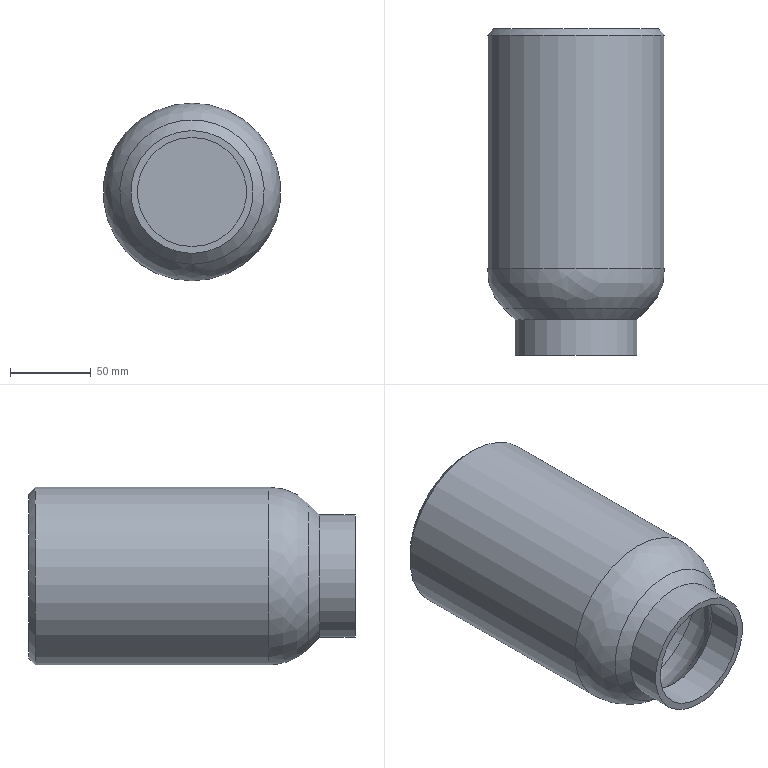Part | NX | 2 solids | 15 faces | box 110 x 202 x 110 mm | volume 227376 mm3 | plane 5 | cylinder 4 | cone 4 | spline 2 | commonest cylinder face diameters 67.515 x1 76 x1 104 x1 110 x1
STEP:
#1=CARTESIAN_POINT('',(4712.585,-22.,-359.679));
#2=VERTEX_POINT('',#1);
#3=CARTESIAN_POINT('',(4712.585,-22.,-321.679));
#4=DIRECTION('',(0.,-1.,0.));
#5=DIRECTION('',(0.,0.,-1.));
#6=AXIS2_PLACEMENT_3D('',#3,#4,#5);
#7=CIRCLE('',#6,38.);
#8=EDGE_CURVE('',#2,#2,#7,.T.);
#9=ORIENTED_EDGE('',*,*,#8,.F.);
#10=EDGE_LOOP('',(#9));
#11=FACE_BOUND('',#10,.T.);
#12=CARTESIAN_POINT('',(4712.585,0.,-359.679));
#13=VERTEX_POINT('',#12);
#14=CARTESIAN_POINT('',(4712.585,0.,-321.679));
#15=DIRECTION('',(0.,-1.,0.));
#16=DIRECTION('',(0.,0.,-1.));
#17=AXIS2_PLACEMENT_3D('',#14,#15,#16);
#18=CIRCLE('',#17,38.);
#19=EDGE_CURVE('',#13,#13,#18,.T.);
#20=ORIENTED_EDGE('',*,*,#19,.T.);
#21=EDGE_LOOP('',(#20));
#22=FACE_BOUND('',#21,.T.);
#23=CARTESIAN_POINT('',(4712.585,-22.,-321.679));
#24=DIRECTION('',(0.,1.,0.));
#25=DIRECTION('',(0.,0.,1.));
#26=AXIS2_PLACEMENT_3D('',#23,#24,#25);
#27=CYLINDRICAL_SURFACE('',#26,38.);
#28=ADVANCED_FACE('',(#11,#22),#27,.T.);
#29=CARTESIAN_POINT('',(4712.585,-22.,-355.436));
#30=VERTEX_POINT('',#29);
#31=CARTESIAN_POINT('',(4712.585,-22.,-321.679));
#32=DIRECTION('',(0.,-1.,0.));
#33=DIRECTION('',(0.,0.,-1.));
#34=AXIS2_PLACEMENT_3D('',#31,#32,#33);
#35=CIRCLE('',#34,33.757);
#36=EDGE_CURVE('',#30,#30,#35,.T.);
#37=ORIENTED_EDGE('',*,*,#36,.T.);
#38=EDGE_LOOP('',(#37));
#39=FACE_BOUND('',#38,.T.);
#40=CARTESIAN_POINT('',(4712.585,0.,-355.436));
#41=VERTEX_POINT('',#40);
#42=CARTESIAN_POINT('',(4712.585,0.,-321.679));
#43=DIRECTION('',(0.,-1.,0.));
#44=DIRECTION('',(0.,0.,-1.));
#45=AXIS2_PLACEMENT_3D('',#42,#43,#44);
#46=CIRCLE('',#45,33.757);
#47=EDGE_CURVE('',#41,#41,#46,.T.);
#48=ORIENTED_EDGE('',*,*,#47,.F.);
#49=EDGE_LOOP('',(#48));
#50=FACE_BOUND('',#49,.T.);
#51=CARTESIAN_POINT('',(4712.585,-22.,-321.679));
#52=DIRECTION('',(0.,1.,0.));
#53=DIRECTION('',(0.,0.,1.));
#54=AXIS2_PLACEMENT_3D('',#51,#52,#53);
#55=CYLINDRICAL_SURFACE('',#54,33.757);
#56=ADVANCED_FACE('',(#39,#50),#55,.F.);
#57=ORIENTED_EDGE('',*,*,#8,.T.);
#58=EDGE_LOOP('',(#57));
#59=FACE_BOUND('',#58,.T.);
#60=ORIENTED_EDGE('',*,*,#36,.F.);
#61=EDGE_LOOP('',(#60));
#62=FACE_BOUND('',#61,.T.);
#63=CARTESIAN_POINT('',(4712.585,-22.,-321.679));
#64=DIRECTION('',(0.,-1.,0.));
#65=DIRECTION('',(0.,0.,-1.));
#66=AXIS2_PLACEMENT_3D('',#63,#64,#65);
#67=PLANE('',#66);
#68=ADVANCED_FACE('',(#59,#62),#67,.T.);
#69=ORIENTED_EDGE('',*,*,#19,.F.);
#70=EDGE_LOOP('',(#69));
#71=FACE_BOUND('',#70,.T.);
#72=ORIENTED_EDGE('',*,*,#47,.T.);
#73=EDGE_LOOP('',(#72));
#74=FACE_BOUND('',#73,.T.);
#75=CARTESIAN_POINT('',(4712.585,0.,-321.679));
#76=DIRECTION('',(0.,-1.,0.));
#77=DIRECTION('',(0.,0.,-1.));
#78=AXIS2_PLACEMENT_3D('',#75,#76,#77);
#79=PLANE('',#78);
#80=ADVANCED_FACE('',(#71,#74),#79,.F.);
#81=CLOSED_SHELL('',(#28,#56,#68,#80));
#82=MANIFOLD_SOLID_BREP('',#81);
#83=CARTESIAN_POINT('',(4712.585,176.,-376.679));
#84=VERTEX_POINT('',#83);
#85=CARTESIAN_POINT('',(4712.585,176.,-321.679));
#86=DIRECTION('',(0.,-1.,0.));
#87=DIRECTION('',(0.,0.,-1.));
#88=AXIS2_PLACEMENT_3D('',#85,#86,#87);
#89=CIRCLE('',#88,55.);
#90=EDGE_CURVE('',#84,#84,#89,.T.);
#91=ORIENTED_EDGE('',*,*,#90,.T.);
#92=EDGE_LOOP('',(#91));
#93=FACE_BOUND('',#92,.T.);
#94=CARTESIAN_POINT('',(4712.585,31.497,-376.679));
#95=VERTEX_POINT('',#94);
#96=CARTESIAN_POINT('',(4712.585,31.497,-321.679));
#97=DIRECTION('',(0.,1.,0.));
#98=DIRECTION('',(0.,0.,-1.));
#99=AXIS2_PLACEMENT_3D('',#96,#97,#98);
#100=CIRCLE('',#99,55.);
#101=EDGE_CURVE('',#95,#95,#100,.T.);
#102=ORIENTED_EDGE('',*,*,#101,.T.);
#103=EDGE_LOOP('',(#102));
#104=FACE_BOUND('',#103,.T.);
#105=CARTESIAN_POINT('',(4712.585,180.,-321.679));
#106=DIRECTION('',(0.,-1.,0.));
#107=DIRECTION('',(0.,0.,-1.));
#108=AXIS2_PLACEMENT_3D('',#105,#106,#107);
#109=CYLINDRICAL_SURFACE('',#108,55.);
#110=ADVANCED_FACE('',(#93,#104),#109,.T.);
#111=CARTESIAN_POINT('',(4712.585,180.,-372.679));
#112=VERTEX_POINT('',#111);
#113=CARTESIAN_POINT('',(4712.585,180.,-321.679));
#114=DIRECTION('',(0.,1.,0.));
#115=DIRECTION('',(0.,0.,-1.));
#116=AXIS2_PLACEMENT_3D('',#113,#114,#115);
#117=CIRCLE('',#116,51.);
#118=EDGE_CURVE('',#112,#112,#117,.T.);
#119=ORIENTED_EDGE('',*,*,#118,.T.);
#120=EDGE_LOOP('',(#119));
#121=FACE_OUTER_BOUND('',#120,.T.);
#122=CARTESIAN_POINT('',(4712.585,180.,-321.679));
#123=DIRECTION('',(0.,-1.,0.));
#124=DIRECTION('',(0.,0.,-1.));
#125=AXIS2_PLACEMENT_3D('',#122,#123,#124);
#126=PLANE('',#125);
#127=ADVANCED_FACE('',(#121),#126,.F.);
#128=CARTESIAN_POINT('',(4712.585,0.,-355.436));
#129=VERTEX_POINT('',#128);
#130=CARTESIAN_POINT('',(4712.585,0.,-321.679));
#131=DIRECTION('',(0.,-1.,0.));
#132=DIRECTION('',(0.,0.,-1.));
#133=AXIS2_PLACEMENT_3D('',#130,#131,#132);
#134=CIRCLE('',#133,33.757);
#135=EDGE_CURVE('',#129,#129,#134,.T.);
#136=ORIENTED_EDGE('',*,*,#135,.F.);
#137=EDGE_LOOP('',(#136));
#138=FACE_BOUND('',#137,.T.);
#139=CARTESIAN_POINT('',(4712.585,0.,-359.679));
#140=VERTEX_POINT('',#139);
#141=CARTESIAN_POINT('',(4712.585,0.,-321.679));
#142=DIRECTION('',(0.,-1.,0.));
#143=DIRECTION('',(0.,0.,-1.));
#144=AXIS2_PLACEMENT_3D('',#141,#142,#143);
#145=CIRCLE('',#144,38.);
#146=EDGE_CURVE('',#140,#140,#145,.T.);
#147=ORIENTED_EDGE('',*,*,#146,.T.);
#148=EDGE_LOOP('',(#147));
#149=FACE_BOUND('',#148,.T.);
#150=CARTESIAN_POINT('',(4712.585,0.,-321.679));
#151=DIRECTION('',(0.,-1.,0.));
#152=DIRECTION('',(0.,0.,-1.));
#153=AXIS2_PLACEMENT_3D('',#150,#151,#152);
#154=PLANE('',#153);
#155=ADVANCED_FACE('',(#138,#149),#154,.T.);
#156=CARTESIAN_POINT('',(4712.585,6.749,-366.428));
#157=VERTEX_POINT('',#156);
#158=CARTESIAN_POINT('',(4712.585,6.749,-321.679));
#159=DIRECTION('',(0.,-1.,0.));
#160=DIRECTION('',(0.,0.,-1.));
#161=AXIS2_PLACEMENT_3D('',#158,#159,#160);
#162=CIRCLE('',#161,44.749);
#163=EDGE_CURVE('',#157,#157,#162,.T.);
#164=ORIENTED_EDGE('',*,*,#163,.T.);
#165=EDGE_LOOP('',(#164));
#166=FACE_BOUND('',#165,.T.);
#167=ORIENTED_EDGE('',*,*,#146,.F.);
#168=EDGE_LOOP('',(#167));
#169=FACE_BOUND('',#168,.T.);
#170=CARTESIAN_POINT('',(4712.585,0.,-321.679));
#171=DIRECTION('',(0.,1.,0.));
#172=DIRECTION('',(0.,0.,1.));
#173=AXIS2_PLACEMENT_3D('',#170,#171,#172);
#174=CONICAL_SURFACE('',#173,38.,45.);
#175=ADVANCED_FACE('',(#166,#169),#174,.T.);
#176=ORIENTED_EDGE('',*,*,#163,.F.);
#177=EDGE_LOOP('',(#176));
#178=FACE_BOUND('',#177,.T.);
#179=ORIENTED_EDGE('',*,*,#101,.F.);
#180=EDGE_LOOP('',(#179));
#181=FACE_BOUND('',#180,.T.);
#182=CARTESIAN_POINT('',(4712.585,6.749,-366.428));
#183=CARTESIAN_POINT('',(4802.082,6.749,-366.428));
#184=CARTESIAN_POINT('',(4802.082,6.749,-276.93));
#185=CARTESIAN_POINT('',(4712.585,6.749,-276.93));
#186=CARTESIAN_POINT('',(4623.087,6.749,-276.93));
#187=CARTESIAN_POINT('',(4623.087,6.749,-366.428));
#188=CARTESIAN_POINT('',(4712.585,6.749,-366.428));
#189=CARTESIAN_POINT('',(4712.585,13.4,-373.079));
#190=CARTESIAN_POINT('',(4815.385,13.4,-373.079));
#191=CARTESIAN_POINT('',(4815.385,13.4,-270.279));
#192=CARTESIAN_POINT('',(4712.585,13.4,-270.279));
#193=CARTESIAN_POINT('',(4609.784,13.4,-270.279));
#194=CARTESIAN_POINT('',(4609.784,13.4,-373.079));
#195=CARTESIAN_POINT('',(4712.585,13.4,-373.079));
#196=CARTESIAN_POINT('',(4712.585,22.091,-376.679));
#197=CARTESIAN_POINT('',(4822.585,22.091,-376.679));
#198=CARTESIAN_POINT('',(4822.585,22.091,-266.679));
#199=CARTESIAN_POINT('',(4712.585,22.091,-266.679));
#200=CARTESIAN_POINT('',(4602.585,22.091,-266.679));
#201=CARTESIAN_POINT('',(4602.585,22.091,-376.679));
#202=CARTESIAN_POINT('',(4712.585,22.091,-376.679));
#203=CARTESIAN_POINT('',(4712.585,31.497,-376.679));
#204=CARTESIAN_POINT('',(4822.585,31.497,-376.679));
#205=CARTESIAN_POINT('',(4822.585,31.497,-266.679));
#206=CARTESIAN_POINT('',(4712.585,31.497,-266.679));
#207=CARTESIAN_POINT('',(4602.585,31.497,-266.679));
#208=CARTESIAN_POINT('',(4602.585,31.497,-376.679));
#209=CARTESIAN_POINT('',(4712.585,31.497,-376.679));
#210=(BOUNDED_SURFACE()B_SPLINE_SURFACE(3,3,((#182,#183,#184,#185,#186,#187,#188),(#189,#190,#191,#192,#193,#194,#195),(#196,#197,#198,#199,#200,#201,#202),(#203,#204,#205,#206,#207,#208,#209)),.UNSPECIFIED.,.F.,.T.,.F.)B_SPLINE_SURFACE_WITH_KNOTS((4,4),(1,3,3,3,1),(0.,1.),(-0.5,0.,0.5,1.,1.5),.UNSPECIFIED.)GEOMETRIC_REPRESENTATION_ITEM()RATIONAL_B_SPLINE_SURFACE(((1.,0.3333,0.3333,1.,0.3333,0.3333,1.),(0.9493,0.3164,0.3164,0.9493,0.3164,0.3164,0.9493),(0.9493,0.3164,0.3164,0.9493,0.3164,0.3164,0.9493),(1.,0.3333,0.3333,1.,0.3333,0.3333,1.)))REPRESENTATION_ITEM('')SURFACE());
#211=ADVANCED_FACE('',(#178,#181),#210,.T.);
#212=ORIENTED_EDGE('',*,*,#118,.F.);
#213=EDGE_LOOP('',(#212));
#214=FACE_BOUND('',#213,.T.);
#215=ORIENTED_EDGE('',*,*,#90,.F.);
#216=EDGE_LOOP('',(#215));
#217=FACE_BOUND('',#216,.T.);
#218=CARTESIAN_POINT('',(4712.585,176.,-321.679));
#219=DIRECTION('',(0.,-1.,0.));
#220=DIRECTION('',(0.,0.,-1.));
#221=AXIS2_PLACEMENT_3D('',#218,#219,#220);
#222=CONICAL_SURFACE('',#221,55.,45.);
#223=ADVANCED_FACE('',(#214,#217),#222,.T.);
#224=CARTESIAN_POINT('',(4712.585,174.757,-373.679));
#225=VERTEX_POINT('',#224);
#226=CARTESIAN_POINT('',(4712.585,174.757,-321.679));
#227=DIRECTION('',(0.,-1.,0.));
#228=DIRECTION('',(0.,0.,-1.));
#229=AXIS2_PLACEMENT_3D('',#226,#227,#228);
#230=CIRCLE('',#229,52.);
#231=EDGE_CURVE('',#225,#225,#230,.T.);
#232=ORIENTED_EDGE('',*,*,#231,.F.);
#233=EDGE_LOOP('',(#232));
#234=FACE_BOUND('',#233,.T.);
#235=CARTESIAN_POINT('',(4712.585,31.497,-373.679));
#236=VERTEX_POINT('',#235);
#237=CARTESIAN_POINT('',(4712.585,31.497,-321.679));
#238=DIRECTION('',(0.,1.,0.));
#239=DIRECTION('',(0.,0.,-1.));
#240=AXIS2_PLACEMENT_3D('',#237,#238,#239);
#241=CIRCLE('',#240,52.);
#242=EDGE_CURVE('',#236,#236,#241,.T.);
#243=ORIENTED_EDGE('',*,*,#242,.F.);
#244=EDGE_LOOP('',(#243));
#245=FACE_BOUND('',#244,.T.);
#246=CARTESIAN_POINT('',(4712.585,180.,-321.679));
#247=DIRECTION('',(0.,-1.,0.));
#248=DIRECTION('',(0.,0.,-1.));
#249=AXIS2_PLACEMENT_3D('',#246,#247,#248);
#250=CYLINDRICAL_SURFACE('',#249,52.);
#251=ADVANCED_FACE('',(#234,#245),#250,.F.);
#252=CARTESIAN_POINT('',(4712.585,177.,-371.436));
#253=VERTEX_POINT('',#252);
#254=CARTESIAN_POINT('',(4712.585,177.,-321.679));
#255=DIRECTION('',(0.,1.,0.));
#256=DIRECTION('',(0.,0.,-1.));
#257=AXIS2_PLACEMENT_3D('',#254,#255,#256);
#258=CIRCLE('',#257,49.757);
#259=EDGE_CURVE('',#253,#253,#258,.T.);
#260=ORIENTED_EDGE('',*,*,#259,.F.);
#261=EDGE_LOOP('',(#260));
#262=FACE_OUTER_BOUND('',#261,.T.);
#263=CARTESIAN_POINT('',(4712.585,177.,-321.679));
#264=DIRECTION('',(0.,-1.,0.));
#265=DIRECTION('',(0.,0.,-1.));
#266=AXIS2_PLACEMENT_3D('',#263,#264,#265);
#267=PLANE('',#266);
#268=ADVANCED_FACE('',(#262),#267,.T.);
#269=CARTESIAN_POINT('',(4712.585,8.87,-279.051));
#270=VERTEX_POINT('',#269);
#271=CARTESIAN_POINT('',(4712.585,8.87,-321.679));
#272=DIRECTION('',(0.,-1.,0.));
#273=DIRECTION('',(0.,0.,1.));
#274=AXIS2_PLACEMENT_3D('',#271,#272,#273);
#275=CIRCLE('',#274,42.627);
#276=EDGE_CURVE('',#270,#270,#275,.T.);
#277=ORIENTED_EDGE('',*,*,#276,.F.);
#278=EDGE_LOOP('',(#277));
#279=FACE_BOUND('',#278,.T.);
#280=ORIENTED_EDGE('',*,*,#135,.T.);
#281=EDGE_LOOP('',(#280));
#282=FACE_BOUND('',#281,.T.);
#283=CARTESIAN_POINT('',(4712.585,2.121,-321.679));
#284=DIRECTION('',(0.,1.,0.));
#285=DIRECTION('',(0.,0.,1.));
#286=AXIS2_PLACEMENT_3D('',#283,#284,#285);
#287=CONICAL_SURFACE('',#286,35.879,45.);
#288=ADVANCED_FACE('',(#279,#282),#287,.F.);
#289=ORIENTED_EDGE('',*,*,#276,.T.);
#290=EDGE_LOOP('',(#289));
#291=FACE_BOUND('',#290,.T.);
#292=ORIENTED_EDGE('',*,*,#242,.T.);
#293=EDGE_LOOP('',(#292));
#294=FACE_BOUND('',#293,.T.);
#295=CARTESIAN_POINT('',(4712.585,31.497,-373.679));
#296=CARTESIAN_POINT('',(4816.585,31.497,-373.679));
#297=CARTESIAN_POINT('',(4816.585,31.497,-269.679));
#298=CARTESIAN_POINT('',(4712.585,31.497,-269.679));
#299=CARTESIAN_POINT('',(4608.585,31.497,-269.679));
#300=CARTESIAN_POINT('',(4608.585,31.497,-373.679));
#301=CARTESIAN_POINT('',(4712.585,31.497,-373.679));
#302=CARTESIAN_POINT('',(4712.585,22.897,-373.679));
#303=CARTESIAN_POINT('',(4816.585,22.897,-373.679));
#304=CARTESIAN_POINT('',(4816.585,22.897,-269.679));
#305=CARTESIAN_POINT('',(4712.585,22.897,-269.679));
#306=CARTESIAN_POINT('',(4608.585,22.897,-269.679));
#307=CARTESIAN_POINT('',(4608.585,22.897,-373.679));
#308=CARTESIAN_POINT('',(4712.585,22.897,-373.679));
#309=CARTESIAN_POINT('',(4712.585,14.951,-370.388));
#310=CARTESIAN_POINT('',(4810.002,14.951,-370.388));
#311=CARTESIAN_POINT('',(4810.002,14.951,-272.97));
#312=CARTESIAN_POINT('',(4712.585,14.951,-272.97));
#313=CARTESIAN_POINT('',(4615.167,14.951,-272.97));
#314=CARTESIAN_POINT('',(4615.167,14.951,-370.388));
#315=CARTESIAN_POINT('',(4712.585,14.951,-370.388));
#316=CARTESIAN_POINT('',(4712.585,8.87,-364.306));
#317=CARTESIAN_POINT('',(4797.84,8.87,-364.306));
#318=CARTESIAN_POINT('',(4797.84,8.87,-279.051));
#319=CARTESIAN_POINT('',(4712.585,8.87,-279.051));
#320=CARTESIAN_POINT('',(4627.33,8.87,-279.051));
#321=CARTESIAN_POINT('',(4627.33,8.87,-364.306));
#322=CARTESIAN_POINT('',(4712.585,8.87,-364.306));
#323=(BOUNDED_SURFACE()B_SPLINE_SURFACE(3,3,((#295,#296,#297,#298,#299,#300,#301),(#302,#303,#304,#305,#306,#307,#308),(#309,#310,#311,#312,#313,#314,#315),(#316,#317,#318,#319,#320,#321,#322)),.UNSPECIFIED.,.F.,.T.,.F.)B_SPLINE_SURFACE_WITH_KNOTS((4,4),(1,3,3,3,1),(0.,1.),(-0.5,0.,0.5,1.,1.5),.UNSPECIFIED.)GEOMETRIC_REPRESENTATION_ITEM()RATIONAL_B_SPLINE_SURFACE(((1.,0.3333,0.3333,1.,0.3333,0.3333,1.),(0.9493,0.3164,0.3164,0.9493,0.3164,0.3164,0.9493),(0.9493,0.3164,0.3164,0.9493,0.3164,0.3164,0.9493),(1.,0.3333,0.3333,1.,0.3333,0.3333,1.)))REPRESENTATION_ITEM('')SURFACE());
#324=ADVANCED_FACE('',(#291,#294),#323,.T.);
#325=ORIENTED_EDGE('',*,*,#259,.T.);
#326=EDGE_LOOP('',(#325));
#327=FACE_BOUND('',#326,.T.);
#328=ORIENTED_EDGE('',*,*,#231,.T.);
#329=EDGE_LOOP('',(#328));
#330=FACE_BOUND('',#329,.T.);
#331=CARTESIAN_POINT('',(4712.585,173.879,-321.679));
#332=DIRECTION('',(0.,-1.,0.));
#333=DIRECTION('',(0.,0.,-1.));
#334=AXIS2_PLACEMENT_3D('',#331,#332,#333);
#335=CONICAL_SURFACE('',#334,52.879,45.);
#336=ADVANCED_FACE('',(#327,#330),#335,.F.);
#337=CLOSED_SHELL('',(#110,#127,#155,#175,#211,#223,#251,#268,#288,#324,#336));
#338=MANIFOLD_SOLID_BREP('',#337);
#339=(LENGTH_UNIT()NAMED_UNIT(*)SI_UNIT(.MILLI.,.METRE.));
#340=UNCERTAINTY_MEASURE_WITH_UNIT(LENGTH_MEASURE(0.0254),#339,'','');
#341=(NAMED_UNIT(*)PLANE_ANGLE_UNIT()SI_UNIT($,.RADIAN.));
#342=PLANE_ANGLE_MEASURE_WITH_UNIT(PLANE_ANGLE_MEASURE(0.01745),#341);
#343=DIMENSIONAL_EXPONENTS(0.,0.,0.,0.,0.,0.,0.);
#344=(CONVERSION_BASED_UNIT('DEGREE',#342)NAMED_UNIT(#343)PLANE_ANGLE_UNIT());
#345=(NAMED_UNIT(*)SI_UNIT($,.STERADIAN.)SOLID_ANGLE_UNIT());
#346=(GEOMETRIC_REPRESENTATION_CONTEXT(3)GLOBAL_UNCERTAINTY_ASSIGNED_CONTEXT((#340))GLOBAL_UNIT_ASSIGNED_CONTEXT((#339,#344,#345))REPRESENTATION_CONTEXT('',''));
#347=ADVANCED_BREP_SHAPE_REPRESENTATION('',(#82,#338),#346);